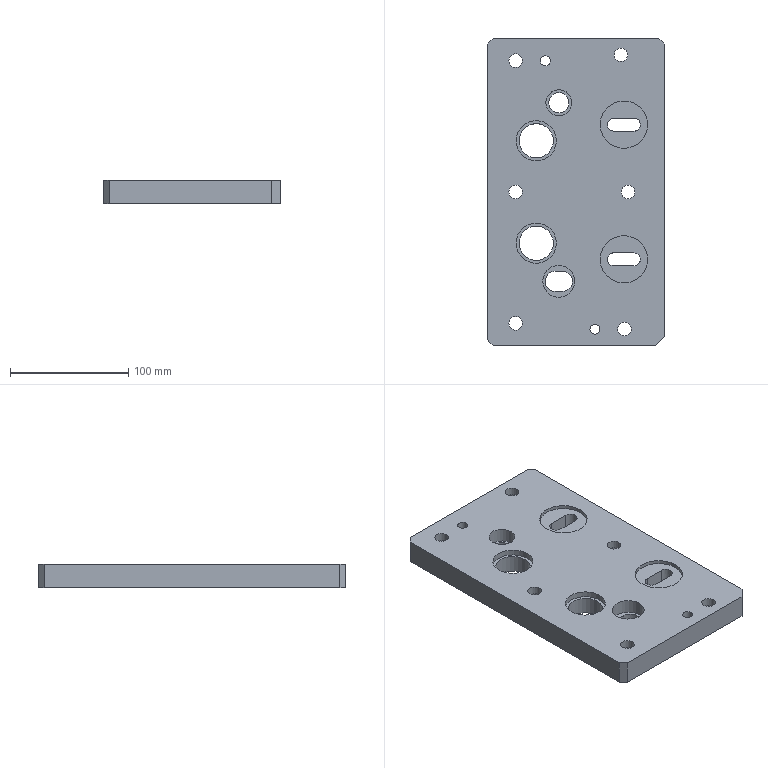Part | STEP file | lll_id3538_x_t | 1 solid | 57 faces | box 150 x 260 x 20 mm | volume 689973 mm3 | plane 28 | cylinder 23 | spline 6 | commonest cylinder face diameters 11.509 x6 18.007 x6 8.505 x2 29.07 x2 34 x2 40 x2